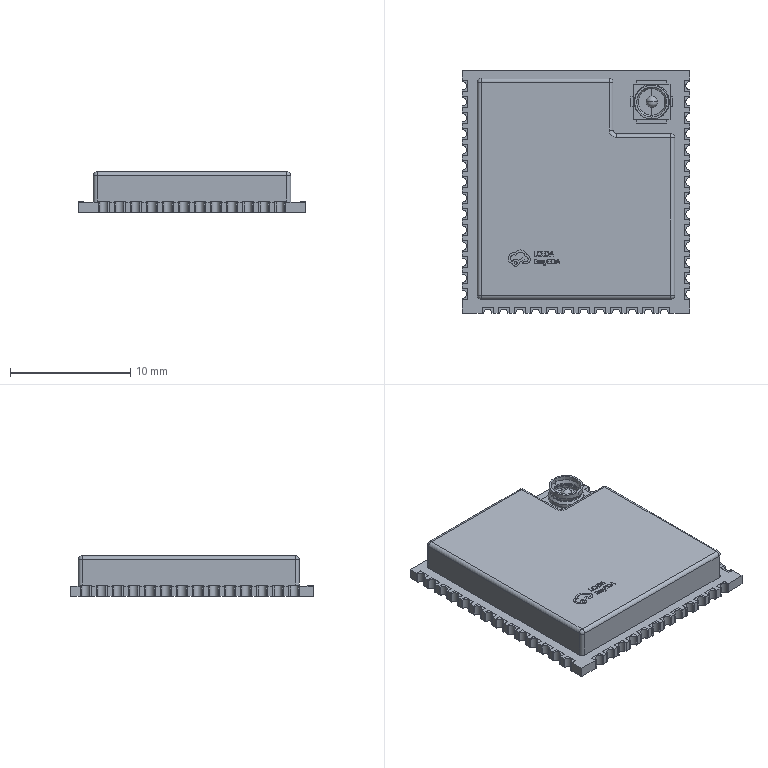Part | NX | features BREP 25 | 25 solids | 894 faces | box 18.88 x 20.127 x 3.364 mm | volume 1016 mm3 | plane 672 | spline 112 | cylinder 68 | cone 22 | torus 13 | sphere 7 | commonest cylinder face diameters 0.681 x54 0.629 x12 0.943 x2